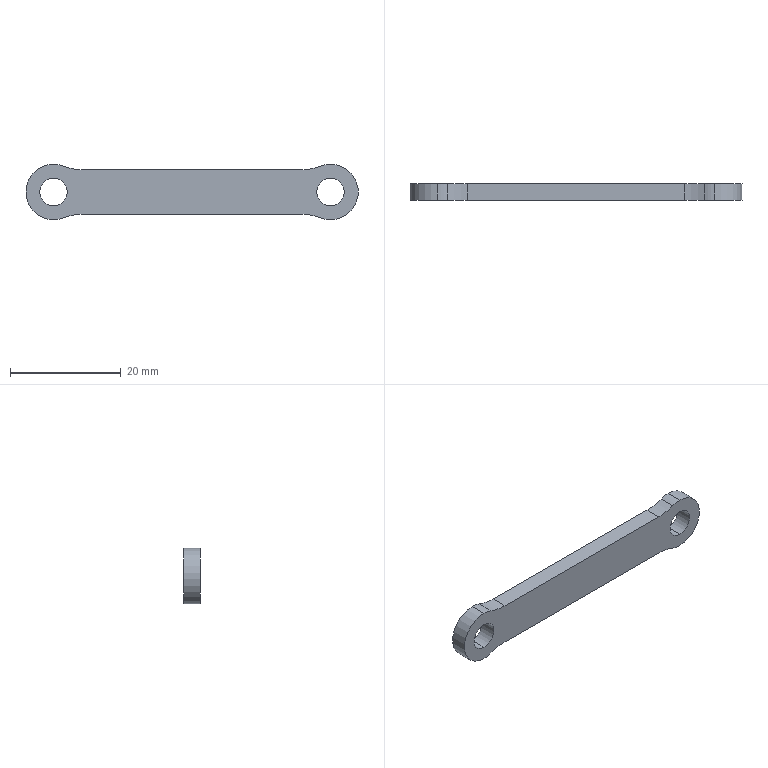Part | SolidWorks | features Extrusion 1, Fillet 1 | 1 solid | 18 faces | box 60 x 3 x 10 mm | volume 1346 mm3 | cylinder 14 | plane 4 | commonest cylinder face diameters 10 x6 5 x4 20 x4
STEP:
#1=CARTESIAN_POINT('',(50.,3.,-2.5));
#2=VERTEX_POINT('',#1);
#3=CARTESIAN_POINT('',(50.,3.,2.5));
#4=VERTEX_POINT('',#3);
#5=CARTESIAN_POINT('',(50.,3.,0.));
#6=DIRECTION('',(0.,1.,0.));
#7=DIRECTION('',(0.,0.,1.));
#8=AXIS2_PLACEMENT_3D('',#5,#6,#7);
#9=CIRCLE('',#8,2.5);
#10=EDGE_CURVE('',#2,#4,#9,.T.);
#11=ORIENTED_EDGE('',*,*,#10,.T.);
#12=CARTESIAN_POINT('',(50.,0.,2.5));
#13=VERTEX_POINT('',#12);
#14=CARTESIAN_POINT('',(50.,3.,2.5));
#15=DIRECTION('',(0.,-1.,0.));
#16=VECTOR('',#15,1000.);
#17=LINE('',#14,#16);
#18=EDGE_CURVE('',#4,#13,#17,.T.);
#19=ORIENTED_EDGE('',*,*,#18,.T.);
#20=CARTESIAN_POINT('',(50.,0.,-2.5));
#21=VERTEX_POINT('',#20);
#22=CARTESIAN_POINT('',(50.,0.,0.));
#23=DIRECTION('',(0.,1.,0.));
#24=DIRECTION('',(0.,0.,1.));
#25=AXIS2_PLACEMENT_3D('',#22,#23,#24);
#26=CIRCLE('',#25,2.5);
#27=EDGE_CURVE('',#21,#13,#26,.T.);
#28=ORIENTED_EDGE('',*,*,#27,.F.);
#29=CARTESIAN_POINT('',(50.,3.,-2.5));
#30=DIRECTION('',(0.,-1.,0.));
#31=VECTOR('',#30,1000.);
#32=LINE('',#29,#31);
#33=EDGE_CURVE('',#2,#21,#32,.T.);
#34=ORIENTED_EDGE('',*,*,#33,.F.);
#35=EDGE_LOOP('',(#11,#19,#28,#34));
#36=FACE_OUTER_BOUND('',#35,.T.);
#37=CARTESIAN_POINT('',(50.,3.,0.));
#38=DIRECTION('',(0.,-1.,0.));
#39=DIRECTION('',(0.,0.,-1.));
#40=AXIS2_PLACEMENT_3D('',#37,#38,#39);
#41=CYLINDRICAL_SURFACE('',#40,2.5);
#42=ADVANCED_FACE('',(#36),#41,.F.);
#43=CARTESIAN_POINT('',(0.,3.,-2.5));
#44=VERTEX_POINT('',#43);
#45=CARTESIAN_POINT('',(0.,3.,2.5));
#46=VERTEX_POINT('',#45);
#47=CARTESIAN_POINT('',(0.,3.,0.));
#48=DIRECTION('',(0.,1.,0.));
#49=DIRECTION('',(0.,0.,1.));
#50=AXIS2_PLACEMENT_3D('',#47,#48,#49);
#51=CIRCLE('',#50,2.5);
#52=EDGE_CURVE('',#44,#46,#51,.T.);
#53=ORIENTED_EDGE('',*,*,#52,.T.);
#54=CARTESIAN_POINT('',(0.,0.,2.5));
#55=VERTEX_POINT('',#54);
#56=CARTESIAN_POINT('',(0.,3.,2.5));
#57=DIRECTION('',(0.,-1.,0.));
#58=VECTOR('',#57,1000.);
#59=LINE('',#56,#58);
#60=EDGE_CURVE('',#46,#55,#59,.T.);
#61=ORIENTED_EDGE('',*,*,#60,.T.);
#62=CARTESIAN_POINT('',(0.,0.,-2.5));
#63=VERTEX_POINT('',#62);
#64=CARTESIAN_POINT('',(0.,0.,0.));
#65=DIRECTION('',(0.,1.,0.));
#66=DIRECTION('',(0.,0.,1.));
#67=AXIS2_PLACEMENT_3D('',#64,#65,#66);
#68=CIRCLE('',#67,2.5);
#69=EDGE_CURVE('',#63,#55,#68,.T.);
#70=ORIENTED_EDGE('',*,*,#69,.F.);
#71=CARTESIAN_POINT('',(0.,3.,-2.5));
#72=DIRECTION('',(0.,-1.,0.));
#73=VECTOR('',#72,1000.);
#74=LINE('',#71,#73);
#75=EDGE_CURVE('',#44,#63,#74,.T.);
#76=ORIENTED_EDGE('',*,*,#75,.F.);
#77=EDGE_LOOP('',(#53,#61,#70,#76));
#78=FACE_OUTER_BOUND('',#77,.T.);
#79=CARTESIAN_POINT('',(0.,3.,0.));
#80=DIRECTION('',(0.,-1.,0.));
#81=DIRECTION('',(0.,0.,-1.));
#82=AXIS2_PLACEMENT_3D('',#79,#80,#81);
#83=CYLINDRICAL_SURFACE('',#82,2.5);
#84=ADVANCED_FACE('',(#78),#83,.F.);
#85=CARTESIAN_POINT('',(50.,3.,5.));
#86=VERTEX_POINT('',#85);
#87=CARTESIAN_POINT('',(50.,3.,-5.));
#88=VERTEX_POINT('',#87);
#89=CARTESIAN_POINT('',(50.,3.,0.));
#90=DIRECTION('',(0.,1.,0.));
#91=DIRECTION('',(0.,0.,1.));
#92=AXIS2_PLACEMENT_3D('',#89,#90,#91);
#93=CIRCLE('',#92,5.);
#94=EDGE_CURVE('',#86,#88,#93,.T.);
#95=ORIENTED_EDGE('',*,*,#94,.F.);
#96=CARTESIAN_POINT('',(50.,0.,5.));
#97=VERTEX_POINT('',#96);
#98=CARTESIAN_POINT('',(50.,3.,5.));
#99=DIRECTION('',(0.,-1.,0.));
#100=VECTOR('',#99,1000.);
#101=LINE('',#98,#100);
#102=EDGE_CURVE('',#86,#97,#101,.T.);
#103=ORIENTED_EDGE('',*,*,#102,.T.);
#104=CARTESIAN_POINT('',(50.,0.,-5.));
#105=VERTEX_POINT('',#104);
#106=CARTESIAN_POINT('',(50.,0.,0.));
#107=DIRECTION('',(0.,1.,0.));
#108=DIRECTION('',(0.,0.,1.));
#109=AXIS2_PLACEMENT_3D('',#106,#107,#108);
#110=CIRCLE('',#109,5.);
#111=EDGE_CURVE('',#97,#105,#110,.T.);
#112=ORIENTED_EDGE('',*,*,#111,.T.);
#113=CARTESIAN_POINT('',(50.,3.,-5.));
#114=DIRECTION('',(0.,-1.,0.));
#115=VECTOR('',#114,1000.);
#116=LINE('',#113,#115);
#117=EDGE_CURVE('',#88,#105,#116,.T.);
#118=ORIENTED_EDGE('',*,*,#117,.F.);
#119=EDGE_LOOP('',(#95,#103,#112,#118));
#120=FACE_OUTER_BOUND('',#119,.T.);
#121=CARTESIAN_POINT('',(50.,3.,0.));
#122=DIRECTION('',(0.,-1.,0.));
#123=DIRECTION('',(0.,0.,-1.));
#124=AXIS2_PLACEMENT_3D('',#121,#122,#123);
#125=CYLINDRICAL_SURFACE('',#124,5.);
#126=ADVANCED_FACE('',(#120),#125,.T.);
#127=CARTESIAN_POINT('',(48.205,3.,-4.667));
#128=VERTEX_POINT('',#127);
#129=CARTESIAN_POINT('',(50.,3.,0.));
#130=DIRECTION('',(0.,1.,0.));
#131=DIRECTION('',(0.,0.,1.));
#132=AXIS2_PLACEMENT_3D('',#129,#130,#131);
#133=CIRCLE('',#132,5.);
#134=EDGE_CURVE('',#88,#128,#133,.T.);
#135=ORIENTED_EDGE('',*,*,#134,.F.);
#136=ORIENTED_EDGE('',*,*,#117,.T.);
#137=CARTESIAN_POINT('',(48.205,0.,-4.667));
#138=VERTEX_POINT('',#137);
#139=CARTESIAN_POINT('',(50.,0.,0.));
#140=DIRECTION('',(0.,1.,0.));
#141=DIRECTION('',(0.,0.,1.));
#142=AXIS2_PLACEMENT_3D('',#139,#140,#141);
#143=CIRCLE('',#142,5.);
#144=EDGE_CURVE('',#105,#138,#143,.T.);
#145=ORIENTED_EDGE('',*,*,#144,.T.);
#146=CARTESIAN_POINT('',(48.205,3.,-4.667));
#147=DIRECTION('',(0.,1.,0.));
#148=VECTOR('',#147,1000.);
#149=LINE('',#146,#148);
#150=EDGE_CURVE('',#138,#128,#149,.T.);
#151=ORIENTED_EDGE('',*,*,#150,.T.);
#152=EDGE_LOOP('',(#135,#136,#145,#151));
#153=FACE_OUTER_BOUND('',#152,.T.);
#154=CARTESIAN_POINT('',(50.,3.,0.));
#155=DIRECTION('',(0.,-1.,0.));
#156=DIRECTION('',(0.,0.,-1.));
#157=AXIS2_PLACEMENT_3D('',#154,#155,#156);
#158=CYLINDRICAL_SURFACE('',#157,5.);
#159=ADVANCED_FACE('',(#153),#158,.T.);
#160=CARTESIAN_POINT('',(0.,3.,5.));
#161=VERTEX_POINT('',#160);
#162=CARTESIAN_POINT('',(1.795,3.,4.667));
#163=VERTEX_POINT('',#162);
#164=CARTESIAN_POINT('',(0.,3.,0.));
#165=DIRECTION('',(0.,1.,0.));
#166=DIRECTION('',(0.,0.,1.));
#167=AXIS2_PLACEMENT_3D('',#164,#165,#166);
#168=CIRCLE('',#167,5.);
#169=EDGE_CURVE('',#161,#163,#168,.T.);
#170=ORIENTED_EDGE('',*,*,#169,.F.);
#171=CARTESIAN_POINT('',(0.,0.,5.));
#172=VERTEX_POINT('',#171);
#173=CARTESIAN_POINT('',(0.,3.,5.));
#174=DIRECTION('',(0.,-1.,0.));
#175=VECTOR('',#174,1000.);
#176=LINE('',#173,#175);
#177=EDGE_CURVE('',#161,#172,#176,.T.);
#178=ORIENTED_EDGE('',*,*,#177,.T.);
#179=CARTESIAN_POINT('',(1.795,0.,4.667));
#180=VERTEX_POINT('',#179);
#181=CARTESIAN_POINT('',(0.,0.,0.));
#182=DIRECTION('',(0.,1.,0.));
#183=DIRECTION('',(0.,0.,1.));
#184=AXIS2_PLACEMENT_3D('',#181,#182,#183);
#185=CIRCLE('',#184,5.);
#186=EDGE_CURVE('',#172,#180,#185,.T.);
#187=ORIENTED_EDGE('',*,*,#186,.T.);
#188=CARTESIAN_POINT('',(1.795,3.,4.667));
#189=DIRECTION('',(0.,1.,0.));
#190=VECTOR('',#189,1000.);
#191=LINE('',#188,#190);
#192=EDGE_CURVE('',#180,#163,#191,.T.);
#193=ORIENTED_EDGE('',*,*,#192,.T.);
#194=EDGE_LOOP('',(#170,#178,#187,#193));
#195=FACE_OUTER_BOUND('',#194,.T.);
#196=CARTESIAN_POINT('',(0.,3.,0.));
#197=DIRECTION('',(0.,-1.,0.));
#198=DIRECTION('',(0.,0.,-1.));
#199=AXIS2_PLACEMENT_3D('',#196,#197,#198);
#200=CYLINDRICAL_SURFACE('',#199,5.);
#201=ADVANCED_FACE('',(#195),#200,.T.);
#202=ORIENTED_EDGE('',*,*,#177,.F.);
#203=CARTESIAN_POINT('',(0.,3.,-5.));
#204=VERTEX_POINT('',#203);
#205=CARTESIAN_POINT('',(0.,3.,0.));
#206=DIRECTION('',(0.,1.,0.));
#207=DIRECTION('',(0.,0.,1.));
#208=AXIS2_PLACEMENT_3D('',#205,#206,#207);
#209=CIRCLE('',#208,5.);
#210=EDGE_CURVE('',#204,#161,#209,.T.);
#211=ORIENTED_EDGE('',*,*,#210,.F.);
#212=CARTESIAN_POINT('',(0.,0.,-5.));
#213=VERTEX_POINT('',#212);
#214=CARTESIAN_POINT('',(0.,3.,-5.));
#215=DIRECTION('',(0.,-1.,0.));
#216=VECTOR('',#215,1000.);
#217=LINE('',#214,#216);
#218=EDGE_CURVE('',#204,#213,#217,.T.);
#219=ORIENTED_EDGE('',*,*,#218,.T.);
#220=CARTESIAN_POINT('',(0.,0.,0.));
#221=DIRECTION('',(0.,1.,0.));
#222=DIRECTION('',(0.,0.,1.));
#223=AXIS2_PLACEMENT_3D('',#220,#221,#222);
#224=CIRCLE('',#223,5.);
#225=EDGE_CURVE('',#213,#172,#224,.T.);
#226=ORIENTED_EDGE('',*,*,#225,.T.);
#227=EDGE_LOOP('',(#202,#211,#219,#226));
#228=FACE_OUTER_BOUND('',#227,.T.);
#229=CARTESIAN_POINT('',(0.,3.,0.));
#230=DIRECTION('',(0.,-1.,0.));
#231=DIRECTION('',(0.,0.,-1.));
#232=AXIS2_PLACEMENT_3D('',#229,#230,#231);
#233=CYLINDRICAL_SURFACE('',#232,5.);
#234=ADVANCED_FACE('',(#228),#233,.T.);
#235=ORIENTED_EDGE('',*,*,#52,.F.);
#236=CARTESIAN_POINT('',(0.,3.,0.));
#237=DIRECTION('',(0.,1.,0.));
#238=DIRECTION('',(0.,0.,1.));
#239=AXIS2_PLACEMENT_3D('',#236,#237,#238);
#240=CIRCLE('',#239,2.5);
#241=EDGE_CURVE('',#46,#44,#240,.T.);
#242=ORIENTED_EDGE('',*,*,#241,.F.);
#243=EDGE_LOOP('',(#235,#242));
#244=FACE_BOUND('',#243,.T.);
#245=CARTESIAN_POINT('',(44.615,3.,-4.));
#246=VERTEX_POINT('',#245);
#247=CARTESIAN_POINT('',(5.385,3.,-4.));
#248=VERTEX_POINT('',#247);
#249=CARTESIAN_POINT('',(3.,3.,-4.));
#250=DIRECTION('',(-1.,0.,0.));
#251=VECTOR('',#250,1000.);
#252=LINE('',#249,#251);
#253=EDGE_CURVE('',#246,#248,#252,.T.);
#254=ORIENTED_EDGE('',*,*,#253,.T.);
#255=CARTESIAN_POINT('',(1.795,3.,-4.667));
#256=VERTEX_POINT('',#255);
#257=CARTESIAN_POINT('',(5.385,3.,-14.));
#258=DIRECTION('',(0.,-1.,0.));
#259=DIRECTION('',(0.,0.,1.));
#260=AXIS2_PLACEMENT_3D('',#257,#258,#259);
#261=CIRCLE('',#260,10.);
#262=EDGE_CURVE('',#248,#256,#261,.T.);
#263=ORIENTED_EDGE('',*,*,#262,.T.);
#264=CARTESIAN_POINT('',(0.,3.,0.));
#265=DIRECTION('',(0.,1.,0.));
#266=DIRECTION('',(0.,0.,1.));
#267=AXIS2_PLACEMENT_3D('',#264,#265,#266);
#268=CIRCLE('',#267,5.);
#269=EDGE_CURVE('',#256,#204,#268,.T.);
#270=ORIENTED_EDGE('',*,*,#269,.T.);
#271=ORIENTED_EDGE('',*,*,#210,.T.);
#272=ORIENTED_EDGE('',*,*,#169,.T.);
#273=CARTESIAN_POINT('',(5.385,3.,4.));
#274=VERTEX_POINT('',#273);
#275=CARTESIAN_POINT('',(5.385,3.,14.));
#276=DIRECTION('',(0.,-1.,0.));
#277=DIRECTION('',(0.,0.,1.));
#278=AXIS2_PLACEMENT_3D('',#275,#276,#277);
#279=CIRCLE('',#278,10.);
#280=EDGE_CURVE('',#163,#274,#279,.T.);
#281=ORIENTED_EDGE('',*,*,#280,.T.);
#282=CARTESIAN_POINT('',(44.615,3.,4.));
#283=VERTEX_POINT('',#282);
#284=CARTESIAN_POINT('',(3.,3.,4.));
#285=DIRECTION('',(1.,0.,0.));
#286=VECTOR('',#285,1000.);
#287=LINE('',#284,#286);
#288=EDGE_CURVE('',#274,#283,#287,.T.);
#289=ORIENTED_EDGE('',*,*,#288,.T.);
#290=CARTESIAN_POINT('',(48.205,3.,4.667));
#291=VERTEX_POINT('',#290);
#292=CARTESIAN_POINT('',(44.615,3.,14.));
#293=DIRECTION('',(0.,-1.,0.));
#294=DIRECTION('',(0.,0.,1.));
#295=AXIS2_PLACEMENT_3D('',#292,#293,#294);
#296=CIRCLE('',#295,10.);
#297=EDGE_CURVE('',#283,#291,#296,.T.);
#298=ORIENTED_EDGE('',*,*,#297,.T.);
#299=CARTESIAN_POINT('',(50.,3.,0.));
#300=DIRECTION('',(0.,1.,0.));
#301=DIRECTION('',(0.,0.,1.));
#302=AXIS2_PLACEMENT_3D('',#299,#300,#301);
#303=CIRCLE('',#302,5.);
#304=EDGE_CURVE('',#291,#86,#303,.T.);
#305=ORIENTED_EDGE('',*,*,#304,.T.);
#306=ORIENTED_EDGE('',*,*,#94,.T.);
#307=ORIENTED_EDGE('',*,*,#134,.T.);
#308=CARTESIAN_POINT('',(44.615,3.,-14.));
#309=DIRECTION('',(0.,-1.,0.));
#310=DIRECTION('',(0.,0.,1.));
#311=AXIS2_PLACEMENT_3D('',#308,#309,#310);
#312=CIRCLE('',#311,10.);
#313=EDGE_CURVE('',#128,#246,#312,.T.);
#314=ORIENTED_EDGE('',*,*,#313,.T.);
#315=EDGE_LOOP('',(#254,#263,#270,#271,#272,#281,#289,#298,#305,#306,#307,#314));
#316=FACE_OUTER_BOUND('',#315,.T.);
#317=ORIENTED_EDGE('',*,*,#10,.F.);
#318=CARTESIAN_POINT('',(50.,3.,0.));
#319=DIRECTION('',(0.,1.,0.));
#320=DIRECTION('',(0.,0.,1.));
#321=AXIS2_PLACEMENT_3D('',#318,#319,#320);
#322=CIRCLE('',#321,2.5);
#323=EDGE_CURVE('',#4,#2,#322,.T.);
#324=ORIENTED_EDGE('',*,*,#323,.F.);
#325=EDGE_LOOP('',(#317,#324));
#326=FACE_BOUND('',#325,.T.);
#327=CARTESIAN_POINT('',(0.,3.,0.));
#328=DIRECTION('',(0.,1.,0.));
#329=DIRECTION('',(0.,0.,1.));
#330=AXIS2_PLACEMENT_3D('',#327,#328,#329);
#331=PLANE('',#330);
#332=ADVANCED_FACE('',(#244,#316,#326),#331,.T.);
#333=CARTESIAN_POINT('',(1.795,0.,-4.667));
#334=VERTEX_POINT('',#333);
#335=CARTESIAN_POINT('',(0.,0.,0.));
#336=DIRECTION('',(0.,1.,0.));
#337=DIRECTION('',(0.,0.,1.));
#338=AXIS2_PLACEMENT_3D('',#335,#336,#337);
#339=CIRCLE('',#338,5.);
#340=EDGE_CURVE('',#334,#213,#339,.T.);
#341=ORIENTED_EDGE('',*,*,#340,.F.);
#342=CARTESIAN_POINT('',(5.385,0.,-4.));
#343=VERTEX_POINT('',#342);
#344=CARTESIAN_POINT('',(5.385,0.,-14.));
#345=DIRECTION('',(0.,1.,0.));
#346=DIRECTION('',(0.,0.,1.));
#347=AXIS2_PLACEMENT_3D('',#344,#345,#346);
#348=CIRCLE('',#347,10.);
#349=EDGE_CURVE('',#334,#343,#348,.T.);
#350=ORIENTED_EDGE('',*,*,#349,.T.);
#351=CARTESIAN_POINT('',(44.615,0.,-4.));
#352=VERTEX_POINT('',#351);
#353=CARTESIAN_POINT('',(3.,0.,-4.));
#354=DIRECTION('',(-1.,0.,0.));
#355=VECTOR('',#354,1000.);
#356=LINE('',#353,#355);
#357=EDGE_CURVE('',#352,#343,#356,.T.);
#358=ORIENTED_EDGE('',*,*,#357,.F.);
#359=CARTESIAN_POINT('',(44.615,0.,-14.));
#360=DIRECTION('',(0.,1.,0.));
#361=DIRECTION('',(0.,0.,1.));
#362=AXIS2_PLACEMENT_3D('',#359,#360,#361);
#363=CIRCLE('',#362,10.);
#364=EDGE_CURVE('',#352,#138,#363,.T.);
#365=ORIENTED_EDGE('',*,*,#364,.T.);
#366=ORIENTED_EDGE('',*,*,#144,.F.);
#367=ORIENTED_EDGE('',*,*,#111,.F.);
#368=CARTESIAN_POINT('',(48.205,0.,4.667));
#369=VERTEX_POINT('',#368);
#370=CARTESIAN_POINT('',(50.,0.,0.));
#371=DIRECTION('',(0.,1.,0.));
#372=DIRECTION('',(0.,0.,1.));
#373=AXIS2_PLACEMENT_3D('',#370,#371,#372);
#374=CIRCLE('',#373,5.);
#375=EDGE_CURVE('',#369,#97,#374,.T.);
#376=ORIENTED_EDGE('',*,*,#375,.F.);
#377=CARTESIAN_POINT('',(44.615,0.,4.));
#378=VERTEX_POINT('',#377);
#379=CARTESIAN_POINT('',(44.615,0.,14.));
#380=DIRECTION('',(0.,1.,0.));
#381=DIRECTION('',(0.,0.,1.));
#382=AXIS2_PLACEMENT_3D('',#379,#380,#381);
#383=CIRCLE('',#382,10.);
#384=EDGE_CURVE('',#369,#378,#383,.T.);
#385=ORIENTED_EDGE('',*,*,#384,.T.);
#386=CARTESIAN_POINT('',(5.385,0.,4.));
#387=VERTEX_POINT('',#386);
#388=CARTESIAN_POINT('',(3.,0.,4.));
#389=DIRECTION('',(1.,0.,0.));
#390=VECTOR('',#389,1000.);
#391=LINE('',#388,#390);
#392=EDGE_CURVE('',#387,#378,#391,.T.);
#393=ORIENTED_EDGE('',*,*,#392,.F.);
#394=CARTESIAN_POINT('',(5.385,0.,14.));
#395=DIRECTION('',(0.,1.,0.));
#396=DIRECTION('',(0.,0.,1.));
#397=AXIS2_PLACEMENT_3D('',#394,#395,#396);
#398=CIRCLE('',#397,10.);
#399=EDGE_CURVE('',#387,#180,#398,.T.);
#400=ORIENTED_EDGE('',*,*,#399,.T.);
#401=ORIENTED_EDGE('',*,*,#186,.F.);
#402=ORIENTED_EDGE('',*,*,#225,.F.);
#403=EDGE_LOOP('',(#341,#350,#358,#365,#366,#367,#376,#385,#393,#400,#401,#402));
#404=FACE_OUTER_BOUND('',#403,.T.);
#405=ORIENTED_EDGE('',*,*,#69,.T.);
#406=CARTESIAN_POINT('',(0.,0.,0.));
#407=DIRECTION('',(0.,1.,0.));
#408=DIRECTION('',(0.,0.,1.));
#409=AXIS2_PLACEMENT_3D('',#406,#407,#408);
#410=CIRCLE('',#409,2.5);
#411=EDGE_CURVE('',#55,#63,#410,.T.);
#412=ORIENTED_EDGE('',*,*,#411,.T.);
#413=EDGE_LOOP('',(#405,#412));
#414=FACE_BOUND('',#413,.T.);
#415=ORIENTED_EDGE('',*,*,#27,.T.);
#416=CARTESIAN_POINT('',(50.,0.,0.));
#417=DIRECTION('',(0.,1.,0.));
#418=DIRECTION('',(0.,0.,1.));
#419=AXIS2_PLACEMENT_3D('',#416,#417,#418);
#420=CIRCLE('',#419,2.5);
#421=EDGE_CURVE('',#13,#21,#420,.T.);
#422=ORIENTED_EDGE('',*,*,#421,.T.);
#423=EDGE_LOOP('',(#415,#422));
#424=FACE_BOUND('',#423,.T.);
#425=CARTESIAN_POINT('',(0.,0.,0.));
#426=DIRECTION('',(0.,1.,0.));
#427=DIRECTION('',(0.,0.,1.));
#428=AXIS2_PLACEMENT_3D('',#425,#426,#427);
#429=PLANE('',#428);
#430=ADVANCED_FACE('',(#404,#414,#424),#429,.F.);
#431=ORIENTED_EDGE('',*,*,#218,.F.);
#432=ORIENTED_EDGE('',*,*,#269,.F.);
#433=CARTESIAN_POINT('',(1.795,3.,-4.667));
#434=DIRECTION('',(0.,-1.,0.));
#435=VECTOR('',#434,1000.);
#436=LINE('',#433,#435);
#437=EDGE_CURVE('',#256,#334,#436,.T.);
#438=ORIENTED_EDGE('',*,*,#437,.T.);
#439=ORIENTED_EDGE('',*,*,#340,.T.);
#440=EDGE_LOOP('',(#431,#432,#438,#439));
#441=FACE_OUTER_BOUND('',#440,.T.);
#442=CARTESIAN_POINT('',(0.,3.,0.));
#443=DIRECTION('',(0.,-1.,0.));
#444=DIRECTION('',(0.,0.,-1.));
#445=AXIS2_PLACEMENT_3D('',#442,#443,#444);
#446=CYLINDRICAL_SURFACE('',#445,5.);
#447=ADVANCED_FACE('',(#441),#446,.T.);
#448=ORIENTED_EDGE('',*,*,#392,.T.);
#449=CARTESIAN_POINT('',(44.615,3.,4.));
#450=DIRECTION('',(0.,1.,0.));
#451=VECTOR('',#450,1000.);
#452=LINE('',#449,#451);
#453=EDGE_CURVE('',#378,#283,#452,.T.);
#454=ORIENTED_EDGE('',*,*,#453,.T.);
#455=ORIENTED_EDGE('',*,*,#288,.F.);
#456=CARTESIAN_POINT('',(5.385,0.,4.));
#457=DIRECTION('',(0.,-1.,0.));
#458=VECTOR('',#457,1000.);
#459=LINE('',#456,#458);
#460=EDGE_CURVE('',#274,#387,#459,.T.);
#461=ORIENTED_EDGE('',*,*,#460,.T.);
#462=EDGE_LOOP('',(#448,#454,#455,#461));
#463=FACE_OUTER_BOUND('',#462,.T.);
#464=CARTESIAN_POINT('',(3.,3.,4.));
#465=DIRECTION('',(0.,0.,-1.));
#466=DIRECTION('',(-1.,0.,0.));
#467=AXIS2_PLACEMENT_3D('',#464,#465,#466);
#468=PLANE('',#467);
#469=ADVANCED_FACE('',(#463),#468,.F.);
#470=ORIENTED_EDGE('',*,*,#102,.F.);
#471=ORIENTED_EDGE('',*,*,#304,.F.);
#472=CARTESIAN_POINT('',(48.205,3.,4.667));
#473=DIRECTION('',(0.,-1.,0.));
#474=VECTOR('',#473,1000.);
#475=LINE('',#472,#474);
#476=EDGE_CURVE('',#291,#369,#475,.T.);
#477=ORIENTED_EDGE('',*,*,#476,.T.);
#478=ORIENTED_EDGE('',*,*,#375,.T.);
#479=EDGE_LOOP('',(#470,#471,#477,#478));
#480=FACE_OUTER_BOUND('',#479,.T.);
#481=CARTESIAN_POINT('',(50.,3.,0.));
#482=DIRECTION('',(0.,-1.,0.));
#483=DIRECTION('',(0.,0.,-1.));
#484=AXIS2_PLACEMENT_3D('',#481,#482,#483);
#485=CYLINDRICAL_SURFACE('',#484,5.);
#486=ADVANCED_FACE('',(#480),#485,.T.);
#487=ORIENTED_EDGE('',*,*,#357,.T.);
#488=CARTESIAN_POINT('',(5.385,3.,-4.));
#489=DIRECTION('',(0.,1.,0.));
#490=VECTOR('',#489,1000.);
#491=LINE('',#488,#490);
#492=EDGE_CURVE('',#343,#248,#491,.T.);
#493=ORIENTED_EDGE('',*,*,#492,.T.);
#494=ORIENTED_EDGE('',*,*,#253,.F.);
#495=CARTESIAN_POINT('',(44.615,0.,-4.));
#496=DIRECTION('',(0.,-1.,0.));
#497=VECTOR('',#496,1000.);
#498=LINE('',#495,#497);
#499=EDGE_CURVE('',#246,#352,#498,.T.);
#500=ORIENTED_EDGE('',*,*,#499,.T.);
#501=EDGE_LOOP('',(#487,#493,#494,#500));
#502=FACE_OUTER_BOUND('',#501,.T.);
#503=CARTESIAN_POINT('',(3.,3.,-4.));
#504=DIRECTION('',(0.,0.,1.));
#505=DIRECTION('',(1.,0.,0.));
#506=AXIS2_PLACEMENT_3D('',#503,#504,#505);
#507=PLANE('',#506);
#508=ADVANCED_FACE('',(#502),#507,.F.);
#509=ORIENTED_EDGE('',*,*,#60,.F.);
#510=ORIENTED_EDGE('',*,*,#241,.T.);
#511=ORIENTED_EDGE('',*,*,#75,.T.);
#512=ORIENTED_EDGE('',*,*,#411,.F.);
#513=EDGE_LOOP('',(#509,#510,#511,#512));
#514=FACE_OUTER_BOUND('',#513,.T.);
#515=CARTESIAN_POINT('',(0.,3.,0.));
#516=DIRECTION('',(0.,-1.,0.));
#517=DIRECTION('',(0.,0.,-1.));
#518=AXIS2_PLACEMENT_3D('',#515,#516,#517);
#519=CYLINDRICAL_SURFACE('',#518,2.5);
#520=ADVANCED_FACE('',(#514),#519,.F.);
#521=ORIENTED_EDGE('',*,*,#18,.F.);
#522=ORIENTED_EDGE('',*,*,#323,.T.);
#523=ORIENTED_EDGE('',*,*,#33,.T.);
#524=ORIENTED_EDGE('',*,*,#421,.F.);
#525=EDGE_LOOP('',(#521,#522,#523,#524));
#526=FACE_OUTER_BOUND('',#525,.T.);
#527=CARTESIAN_POINT('',(50.,3.,0.));
#528=DIRECTION('',(0.,-1.,0.));
#529=DIRECTION('',(0.,0.,-1.));
#530=AXIS2_PLACEMENT_3D('',#527,#528,#529);
#531=CYLINDRICAL_SURFACE('',#530,2.5);
#532=ADVANCED_FACE('',(#526),#531,.F.);
#533=ORIENTED_EDGE('',*,*,#262,.F.);
#534=ORIENTED_EDGE('',*,*,#492,.F.);
#535=ORIENTED_EDGE('',*,*,#349,.F.);
#536=ORIENTED_EDGE('',*,*,#437,.F.);
#537=EDGE_LOOP('',(#533,#534,#535,#536));
#538=FACE_OUTER_BOUND('',#537,.T.);
#539=CARTESIAN_POINT('',(5.385,3.,-14.));
#540=DIRECTION('',(0.,-1.,0.));
#541=DIRECTION('',(0.,0.,-1.));
#542=AXIS2_PLACEMENT_3D('',#539,#540,#541);
#543=CYLINDRICAL_SURFACE('',#542,10.);
#544=ADVANCED_FACE('',(#538),#543,.F.);
#545=ORIENTED_EDGE('',*,*,#313,.F.);
#546=ORIENTED_EDGE('',*,*,#150,.F.);
#547=ORIENTED_EDGE('',*,*,#364,.F.);
#548=ORIENTED_EDGE('',*,*,#499,.F.);
#549=EDGE_LOOP('',(#545,#546,#547,#548));
#550=FACE_OUTER_BOUND('',#549,.T.);
#551=CARTESIAN_POINT('',(44.615,3.,-14.));
#552=DIRECTION('',(0.,-1.,0.));
#553=DIRECTION('',(0.,0.,-1.));
#554=AXIS2_PLACEMENT_3D('',#551,#552,#553);
#555=CYLINDRICAL_SURFACE('',#554,10.);
#556=ADVANCED_FACE('',(#550),#555,.F.);
#557=ORIENTED_EDGE('',*,*,#297,.F.);
#558=ORIENTED_EDGE('',*,*,#453,.F.);
#559=ORIENTED_EDGE('',*,*,#384,.F.);
#560=ORIENTED_EDGE('',*,*,#476,.F.);
#561=EDGE_LOOP('',(#557,#558,#559,#560));
#562=FACE_OUTER_BOUND('',#561,.T.);
#563=CARTESIAN_POINT('',(44.615,3.,14.));
#564=DIRECTION('',(0.,-1.,0.));
#565=DIRECTION('',(0.,0.,-1.));
#566=AXIS2_PLACEMENT_3D('',#563,#564,#565);
#567=CYLINDRICAL_SURFACE('',#566,10.);
#568=ADVANCED_FACE('',(#562),#567,.F.);
#569=ORIENTED_EDGE('',*,*,#280,.F.);
#570=ORIENTED_EDGE('',*,*,#192,.F.);
#571=ORIENTED_EDGE('',*,*,#399,.F.);
#572=ORIENTED_EDGE('',*,*,#460,.F.);
#573=EDGE_LOOP('',(#569,#570,#571,#572));
#574=FACE_OUTER_BOUND('',#573,.T.);
#575=CARTESIAN_POINT('',(5.385,3.,14.));
#576=DIRECTION('',(0.,-1.,0.));
#577=DIRECTION('',(0.,0.,-1.));
#578=AXIS2_PLACEMENT_3D('',#575,#576,#577);
#579=CYLINDRICAL_SURFACE('',#578,10.);
#580=ADVANCED_FACE('',(#574),#579,.F.);
#581=CLOSED_SHELL('',(#42,#84,#126,#159,#201,#234,#332,#430,#447,#469,#486,#508,#520,#532,#544,#556,#568,#580));
#582=MANIFOLD_SOLID_BREP('',#581);
#583=CARTESIAN_POINT('',(0.,0.,0.));
#584=DIRECTION('',(0.,0.,1.));
#585=DIRECTION('',(1.,0.,0.));
#586=AXIS2_PLACEMENT_3D('',#583,#584,#585);
#587=(LENGTH_UNIT()NAMED_UNIT(*)SI_UNIT(.MILLI.,.METRE.));
#588=UNCERTAINTY_MEASURE_WITH_UNIT(LENGTH_MEASURE(0.00001),#587,'','');
#589=(NAMED_UNIT(*)PLANE_ANGLE_UNIT()SI_UNIT($,.RADIAN.));
#590=(NAMED_UNIT(*)SI_UNIT($,.STERADIAN.)SOLID_ANGLE_UNIT());
#591=(GEOMETRIC_REPRESENTATION_CONTEXT(3)GLOBAL_UNCERTAINTY_ASSIGNED_CONTEXT((#588))GLOBAL_UNIT_ASSIGNED_CONTEXT((#587,#589,#590))REPRESENTATION_CONTEXT('',''));
#592=ADVANCED_BREP_SHAPE_REPRESENTATION('',(#582,#586),#591);